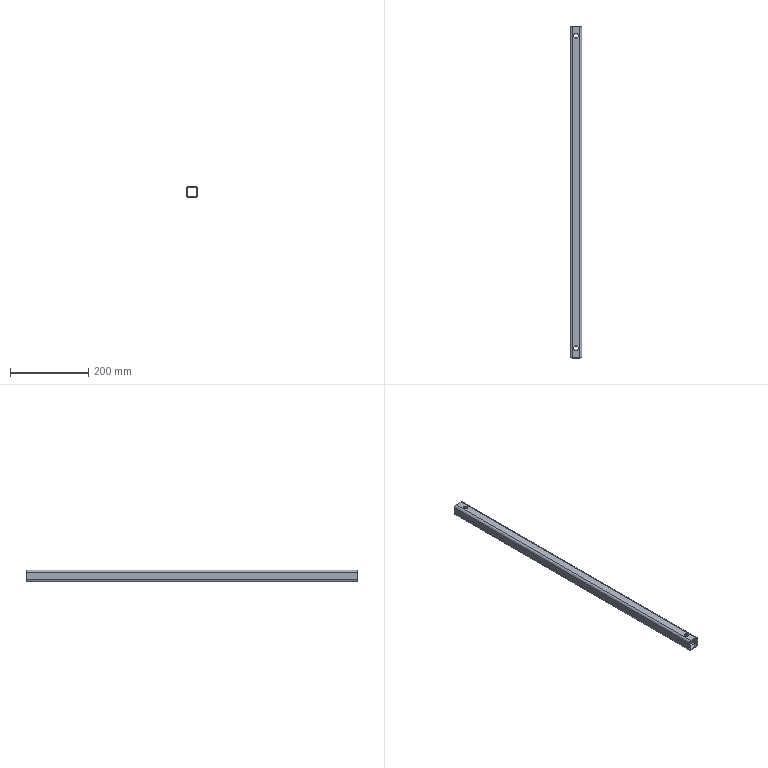Part | NX | features solid 2 | 1 solid | 30 faces | box 30 x 850 x 30 mm | volume 254291 mm3 | cylinder 16 | plane 14 | commonest cylinder face diameters 12 x12 6 x4
STEP:
#1=CARTESIAN_POINT('',(1092.,-720.,1295.));
#2=VERTEX_POINT('',#1);
#3=CARTESIAN_POINT('',(1092.,-720.,1298.));
#4=VERTEX_POINT('',#3);
#5=CARTESIAN_POINT('',(1092.,-720.,1325.));
#6=DIRECTION('',(0.,0.,-1.));
#7=VECTOR('',#6,1000.);
#8=LINE('',#5,#7);
#9=EDGE_CURVE('',#2,#4,#8,.F.);
#10=ORIENTED_EDGE('',*,*,#9,.T.);
#11=CARTESIAN_POINT('',(1104.,-720.,1298.));
#12=VERTEX_POINT('',#11);
#13=CARTESIAN_POINT('',(1098.,-720.,1298.));
#14=DIRECTION('',(0.,0.,-1.));
#15=DIRECTION('',(-1.,0.,0.));
#16=AXIS2_PLACEMENT_3D('',#13,#14,#15);
#17=CIRCLE('',#16,6.);
#18=EDGE_CURVE('',#12,#4,#17,.T.);
#19=ORIENTED_EDGE('',*,*,#18,.F.);
#20=CARTESIAN_POINT('',(1104.,-720.,1295.));
#21=VERTEX_POINT('',#20);
#22=CARTESIAN_POINT('',(1104.,-720.,1325.));
#23=DIRECTION('',(0.,0.,-1.));
#24=VECTOR('',#23,1000.);
#25=LINE('',#22,#24);
#26=EDGE_CURVE('',#12,#21,#25,.T.);
#27=ORIENTED_EDGE('',*,*,#26,.T.);
#28=CARTESIAN_POINT('',(1098.,-720.,1295.));
#29=DIRECTION('',(0.,0.,-1.));
#30=DIRECTION('',(-1.,0.,0.));
#31=AXIS2_PLACEMENT_3D('',#28,#29,#30);
#32=CIRCLE('',#31,6.);
#33=EDGE_CURVE('',#21,#2,#32,.T.);
#34=ORIENTED_EDGE('',*,*,#33,.T.);
#35=EDGE_LOOP('',(#10,#19,#27,#34));
#36=FACE_BOUND('',#35,.T.);
#37=CARTESIAN_POINT('',(1098.,-720.,1325.));
#38=DIRECTION('',(0.,0.,-1.));
#39=DIRECTION('',(1.,0.,0.));
#40=AXIS2_PLACEMENT_3D('',#37,#38,#39);
#41=CYLINDRICAL_SURFACE('',#40,6.);
#42=ADVANCED_FACE('',(#36),#41,.F.);
#43=CARTESIAN_POINT('',(1092.,-720.,1325.));
#44=VERTEX_POINT('',#43);
#45=CARTESIAN_POINT('',(1092.,-720.,1322.));
#46=VERTEX_POINT('',#45);
#47=CARTESIAN_POINT('',(1092.,-720.,1325.));
#48=DIRECTION('',(0.,0.,-1.));
#49=VECTOR('',#48,1000.);
#50=LINE('',#47,#49);
#51=EDGE_CURVE('',#44,#46,#50,.T.);
#52=ORIENTED_EDGE('',*,*,#51,.F.);
#53=CARTESIAN_POINT('',(1104.,-720.,1325.));
#54=VERTEX_POINT('',#53);
#55=CARTESIAN_POINT('',(1098.,-720.,1325.));
#56=DIRECTION('',(0.,0.,-1.));
#57=DIRECTION('',(1.,0.,0.));
#58=AXIS2_PLACEMENT_3D('',#55,#56,#57);
#59=CIRCLE('',#58,6.);
#60=EDGE_CURVE('',#54,#44,#59,.T.);
#61=ORIENTED_EDGE('',*,*,#60,.F.);
#62=CARTESIAN_POINT('',(1104.,-720.,1322.));
#63=VERTEX_POINT('',#62);
#64=CARTESIAN_POINT('',(1104.,-720.,1325.));
#65=DIRECTION('',(0.,0.,-1.));
#66=VECTOR('',#65,1000.);
#67=LINE('',#64,#66);
#68=EDGE_CURVE('',#63,#54,#67,.F.);
#69=ORIENTED_EDGE('',*,*,#68,.F.);
#70=CARTESIAN_POINT('',(1098.,-720.,1322.));
#71=DIRECTION('',(0.,0.,1.));
#72=DIRECTION('',(1.,0.,0.));
#73=AXIS2_PLACEMENT_3D('',#70,#71,#72);
#74=CIRCLE('',#73,6.);
#75=EDGE_CURVE('',#46,#63,#74,.T.);
#76=ORIENTED_EDGE('',*,*,#75,.F.);
#77=EDGE_LOOP('',(#52,#61,#69,#76));
#78=FACE_BOUND('',#77,.T.);
#79=CARTESIAN_POINT('',(1098.,-720.,1325.));
#80=DIRECTION('',(0.,0.,-1.));
#81=DIRECTION('',(1.,0.,0.));
#82=AXIS2_PLACEMENT_3D('',#79,#80,#81);
#83=CYLINDRICAL_SURFACE('',#82,6.);
#84=ADVANCED_FACE('',(#78),#83,.F.);
#85=CARTESIAN_POINT('',(1092.,-1520.,1295.));
#86=VERTEX_POINT('',#85);
#87=CARTESIAN_POINT('',(1092.,-1520.,1298.));
#88=VERTEX_POINT('',#87);
#89=CARTESIAN_POINT('',(1092.,-1520.,1325.));
#90=DIRECTION('',(0.,0.,-1.));
#91=VECTOR('',#90,1000.);
#92=LINE('',#89,#91);
#93=EDGE_CURVE('',#86,#88,#92,.F.);
#94=ORIENTED_EDGE('',*,*,#93,.T.);
#95=CARTESIAN_POINT('',(1104.,-1520.,1298.));
#96=VERTEX_POINT('',#95);
#97=CARTESIAN_POINT('',(1098.,-1520.,1298.));
#98=DIRECTION('',(0.,0.,-1.));
#99=DIRECTION('',(-1.,0.,0.));
#100=AXIS2_PLACEMENT_3D('',#97,#98,#99);
#101=CIRCLE('',#100,6.);
#102=EDGE_CURVE('',#96,#88,#101,.T.);
#103=ORIENTED_EDGE('',*,*,#102,.F.);
#104=CARTESIAN_POINT('',(1104.,-1520.,1295.));
#105=VERTEX_POINT('',#104);
#106=CARTESIAN_POINT('',(1104.,-1520.,1325.));
#107=DIRECTION('',(0.,0.,-1.));
#108=VECTOR('',#107,1000.);
#109=LINE('',#106,#108);
#110=EDGE_CURVE('',#96,#105,#109,.T.);
#111=ORIENTED_EDGE('',*,*,#110,.T.);
#112=CARTESIAN_POINT('',(1098.,-1520.,1295.));
#113=DIRECTION('',(0.,0.,-1.));
#114=DIRECTION('',(-1.,0.,0.));
#115=AXIS2_PLACEMENT_3D('',#112,#113,#114);
#116=CIRCLE('',#115,6.);
#117=EDGE_CURVE('',#105,#86,#116,.T.);
#118=ORIENTED_EDGE('',*,*,#117,.T.);
#119=EDGE_LOOP('',(#94,#103,#111,#118));
#120=FACE_BOUND('',#119,.T.);
#121=CARTESIAN_POINT('',(1098.,-1520.,1325.));
#122=DIRECTION('',(0.,0.,-1.));
#123=DIRECTION('',(1.,0.,0.));
#124=AXIS2_PLACEMENT_3D('',#121,#122,#123);
#125=CYLINDRICAL_SURFACE('',#124,6.);
#126=ADVANCED_FACE('',(#120),#125,.F.);
#127=CARTESIAN_POINT('',(1092.,-1520.,1325.));
#128=VERTEX_POINT('',#127);
#129=CARTESIAN_POINT('',(1092.,-1520.,1322.));
#130=VERTEX_POINT('',#129);
#131=CARTESIAN_POINT('',(1092.,-1520.,1325.));
#132=DIRECTION('',(0.,0.,-1.));
#133=VECTOR('',#132,1000.);
#134=LINE('',#131,#133);
#135=EDGE_CURVE('',#128,#130,#134,.T.);
#136=ORIENTED_EDGE('',*,*,#135,.F.);
#137=CARTESIAN_POINT('',(1104.,-1520.,1325.));
#138=VERTEX_POINT('',#137);
#139=CARTESIAN_POINT('',(1098.,-1520.,1325.));
#140=DIRECTION('',(0.,0.,-1.));
#141=DIRECTION('',(1.,0.,0.));
#142=AXIS2_PLACEMENT_3D('',#139,#140,#141);
#143=CIRCLE('',#142,6.);
#144=EDGE_CURVE('',#138,#128,#143,.T.);
#145=ORIENTED_EDGE('',*,*,#144,.F.);
#146=CARTESIAN_POINT('',(1104.,-1520.,1322.));
#147=VERTEX_POINT('',#146);
#148=CARTESIAN_POINT('',(1104.,-1520.,1325.));
#149=DIRECTION('',(0.,0.,-1.));
#150=VECTOR('',#149,1000.);
#151=LINE('',#148,#150);
#152=EDGE_CURVE('',#147,#138,#151,.F.);
#153=ORIENTED_EDGE('',*,*,#152,.F.);
#154=CARTESIAN_POINT('',(1098.,-1520.,1322.));
#155=DIRECTION('',(0.,0.,1.));
#156=DIRECTION('',(1.,0.,0.));
#157=AXIS2_PLACEMENT_3D('',#154,#155,#156);
#158=CIRCLE('',#157,6.);
#159=EDGE_CURVE('',#130,#147,#158,.T.);
#160=ORIENTED_EDGE('',*,*,#159,.F.);
#161=EDGE_LOOP('',(#136,#145,#153,#160));
#162=FACE_BOUND('',#161,.T.);
#163=CARTESIAN_POINT('',(1098.,-1520.,1325.));
#164=DIRECTION('',(0.,0.,-1.));
#165=DIRECTION('',(1.,0.,0.));
#166=AXIS2_PLACEMENT_3D('',#163,#164,#165);
#167=CYLINDRICAL_SURFACE('',#166,6.);
#168=ADVANCED_FACE('',(#162),#167,.F.);
#169=CARTESIAN_POINT('',(1110.,-695.,1319.));
#170=VERTEX_POINT('',#169);
#171=CARTESIAN_POINT('',(1110.,-695.,1310.01));
#172=VERTEX_POINT('',#171);
#173=CARTESIAN_POINT('',(1110.,-695.,1325.));
#174=DIRECTION('',(0.,0.,-1.));
#175=VECTOR('',#174,1000.);
#176=LINE('',#173,#175);
#177=EDGE_CURVE('',#170,#172,#176,.T.);
#178=ORIENTED_EDGE('',*,*,#177,.T.);
#179=CARTESIAN_POINT('',(1110.,-1545.,1310.01));
#180=VERTEX_POINT('',#179);
#181=CARTESIAN_POINT('',(1110.,-1545.,1310.01));
#182=DIRECTION('',(0.,1.,0.));
#183=VECTOR('',#182,1000.);
#184=LINE('',#181,#183);
#185=EDGE_CURVE('',#180,#172,#184,.T.);
#186=ORIENTED_EDGE('',*,*,#185,.F.);
#187=CARTESIAN_POINT('',(1110.,-1545.,1319.));
#188=VERTEX_POINT('',#187);
#189=CARTESIAN_POINT('',(1110.,-1545.,1325.));
#190=DIRECTION('',(0.,0.,-1.));
#191=VECTOR('',#190,1000.);
#192=LINE('',#189,#191);
#193=EDGE_CURVE('',#188,#180,#192,.T.);
#194=ORIENTED_EDGE('',*,*,#193,.F.);
#195=CARTESIAN_POINT('',(1110.,-1545.,1319.));
#196=DIRECTION('',(0.,1.,0.));
#197=VECTOR('',#196,1000.);
#198=LINE('',#195,#197);
#199=EDGE_CURVE('',#188,#170,#198,.T.);
#200=ORIENTED_EDGE('',*,*,#199,.T.);
#201=EDGE_LOOP('',(#178,#186,#194,#200));
#202=FACE_BOUND('',#201,.T.);
#203=CARTESIAN_POINT('',(1110.,-1545.,1325.));
#204=DIRECTION('',(1.,0.,0.));
#205=DIRECTION('',(0.,0.,-1.));
#206=AXIS2_PLACEMENT_3D('',#203,#204,#205);
#207=PLANE('',#206);
#208=ADVANCED_FACE('',(#202),#207,.F.);
#209=CARTESIAN_POINT('',(1107.,-695.,1322.));
#210=VERTEX_POINT('',#209);
#211=CARTESIAN_POINT('',(1107.,-695.,1319.));
#212=DIRECTION('',(0.,1.,0.));
#213=DIRECTION('',(-1.,0.,0.));
#214=AXIS2_PLACEMENT_3D('',#211,#212,#213);
#215=CIRCLE('',#214,3.);
#216=EDGE_CURVE('',#210,#170,#215,.T.);
#217=ORIENTED_EDGE('',*,*,#216,.T.);
#218=ORIENTED_EDGE('',*,*,#199,.F.);
#219=CARTESIAN_POINT('',(1107.,-1545.,1322.));
#220=VERTEX_POINT('',#219);
#221=CARTESIAN_POINT('',(1107.,-1545.,1319.));
#222=DIRECTION('',(0.,1.,0.));
#223=DIRECTION('',(-1.,0.,0.));
#224=AXIS2_PLACEMENT_3D('',#221,#222,#223);
#225=CIRCLE('',#224,3.);
#226=EDGE_CURVE('',#220,#188,#225,.T.);
#227=ORIENTED_EDGE('',*,*,#226,.F.);
#228=CARTESIAN_POINT('',(1107.,-1545.,1322.));
#229=DIRECTION('',(0.,1.,0.));
#230=VECTOR('',#229,1000.);
#231=LINE('',#228,#230);
#232=EDGE_CURVE('',#220,#210,#231,.T.);
#233=ORIENTED_EDGE('',*,*,#232,.T.);
#234=EDGE_LOOP('',(#217,#218,#227,#233));
#235=FACE_BOUND('',#234,.T.);
#236=CARTESIAN_POINT('',(1107.,-1545.,1319.));
#237=DIRECTION('',(0.,1.,0.));
#238=DIRECTION('',(-1.,0.,0.));
#239=AXIS2_PLACEMENT_3D('',#236,#237,#238);
#240=CYLINDRICAL_SURFACE('',#239,3.);
#241=ADVANCED_FACE('',(#235),#240,.F.);
#242=CARTESIAN_POINT('',(1098.,-1520.,1322.));
#243=DIRECTION('',(0.,0.,1.));
#244=DIRECTION('',(1.,0.,0.));
#245=AXIS2_PLACEMENT_3D('',#242,#243,#244);
#246=CIRCLE('',#245,6.);
#247=EDGE_CURVE('',#147,#130,#246,.T.);
#248=ORIENTED_EDGE('',*,*,#247,.T.);
#249=ORIENTED_EDGE('',*,*,#159,.T.);
#250=EDGE_LOOP('',(#248,#249));
#251=FACE_BOUND('',#250,.T.);
#252=CARTESIAN_POINT('',(1098.,-720.,1322.));
#253=DIRECTION('',(0.,0.,1.));
#254=DIRECTION('',(1.,0.,0.));
#255=AXIS2_PLACEMENT_3D('',#252,#253,#254);
#256=CIRCLE('',#255,6.);
#257=EDGE_CURVE('',#63,#46,#256,.T.);
#258=ORIENTED_EDGE('',*,*,#257,.T.);
#259=ORIENTED_EDGE('',*,*,#75,.T.);
#260=EDGE_LOOP('',(#258,#259));
#261=FACE_BOUND('',#260,.T.);
#262=CARTESIAN_POINT('',(1089.,-695.,1322.));
#263=VERTEX_POINT('',#262);
#264=CARTESIAN_POINT('',(1083.,-695.,1322.));
#265=DIRECTION('',(1.,0.,0.));
#266=VECTOR('',#265,1000.);
#267=LINE('',#264,#266);
#268=EDGE_CURVE('',#263,#210,#267,.T.);
#269=ORIENTED_EDGE('',*,*,#268,.T.);
#270=ORIENTED_EDGE('',*,*,#232,.F.);
#271=CARTESIAN_POINT('',(1089.,-1545.,1322.));
#272=VERTEX_POINT('',#271);
#273=CARTESIAN_POINT('',(1083.,-1545.,1322.));
#274=DIRECTION('',(1.,0.,0.));
#275=VECTOR('',#274,1000.);
#276=LINE('',#273,#275);
#277=EDGE_CURVE('',#272,#220,#276,.T.);
#278=ORIENTED_EDGE('',*,*,#277,.F.);
#279=CARTESIAN_POINT('',(1089.,-1545.,1322.));
#280=DIRECTION('',(0.,1.,0.));
#281=VECTOR('',#280,1000.);
#282=LINE('',#279,#281);
#283=EDGE_CURVE('',#272,#263,#282,.T.);
#284=ORIENTED_EDGE('',*,*,#283,.T.);
#285=EDGE_LOOP('',(#269,#270,#278,#284));
#286=FACE_BOUND('',#285,.T.);
#287=CARTESIAN_POINT('',(1083.,-1545.,1322.));
#288=DIRECTION('',(0.,0.,1.));
#289=DIRECTION('',(1.,0.,0.));
#290=AXIS2_PLACEMENT_3D('',#287,#288,#289);
#291=PLANE('',#290);
#292=ADVANCED_FACE('',(#251,#261,#286),#291,.F.);
#293=CARTESIAN_POINT('',(1086.,-695.,1319.));
#294=VERTEX_POINT('',#293);
#295=CARTESIAN_POINT('',(1089.,-695.,1319.));
#296=DIRECTION('',(0.,1.,0.));
#297=DIRECTION('',(-1.,0.,0.));
#298=AXIS2_PLACEMENT_3D('',#295,#296,#297);
#299=CIRCLE('',#298,3.);
#300=EDGE_CURVE('',#294,#263,#299,.T.);
#301=ORIENTED_EDGE('',*,*,#300,.T.);
#302=ORIENTED_EDGE('',*,*,#283,.F.);
#303=CARTESIAN_POINT('',(1086.,-1545.,1319.));
#304=VERTEX_POINT('',#303);
#305=CARTESIAN_POINT('',(1089.,-1545.,1319.));
#306=DIRECTION('',(0.,1.,0.));
#307=DIRECTION('',(-1.,0.,0.));
#308=AXIS2_PLACEMENT_3D('',#305,#306,#307);
#309=CIRCLE('',#308,3.);
#310=EDGE_CURVE('',#304,#272,#309,.T.);
#311=ORIENTED_EDGE('',*,*,#310,.F.);
#312=CARTESIAN_POINT('',(1086.,-1545.,1319.));
#313=DIRECTION('',(0.,1.,0.));
#314=VECTOR('',#313,1000.);
#315=LINE('',#312,#314);
#316=EDGE_CURVE('',#304,#294,#315,.T.);
#317=ORIENTED_EDGE('',*,*,#316,.T.);
#318=EDGE_LOOP('',(#301,#302,#311,#317));
#319=FACE_BOUND('',#318,.T.);
#320=CARTESIAN_POINT('',(1089.,-1545.,1319.));
#321=DIRECTION('',(0.,1.,0.));
#322=DIRECTION('',(-1.,0.,0.));
#323=AXIS2_PLACEMENT_3D('',#320,#321,#322);
#324=CYLINDRICAL_SURFACE('',#323,3.);
#325=ADVANCED_FACE('',(#319),#324,.F.);
#326=CARTESIAN_POINT('',(1086.,-695.,1301.));
#327=VERTEX_POINT('',#326);
#328=CARTESIAN_POINT('',(1086.,-695.,1295.));
#329=DIRECTION('',(0.,0.,1.));
#330=VECTOR('',#329,1000.);
#331=LINE('',#328,#330);
#332=EDGE_CURVE('',#327,#294,#331,.T.);
#333=ORIENTED_EDGE('',*,*,#332,.T.);
#334=ORIENTED_EDGE('',*,*,#316,.F.);
#335=CARTESIAN_POINT('',(1086.,-1545.,1301.));
#336=VERTEX_POINT('',#335);
#337=CARTESIAN_POINT('',(1086.,-1545.,1295.));
#338=DIRECTION('',(0.,0.,1.));
#339=VECTOR('',#338,1000.);
#340=LINE('',#337,#339);
#341=EDGE_CURVE('',#336,#304,#340,.T.);
#342=ORIENTED_EDGE('',*,*,#341,.F.);
#343=CARTESIAN_POINT('',(1086.,-1545.,1301.));
#344=DIRECTION('',(0.,1.,0.));
#345=VECTOR('',#344,1000.);
#346=LINE('',#343,#345);
#347=EDGE_CURVE('',#336,#327,#346,.T.);
#348=ORIENTED_EDGE('',*,*,#347,.T.);
#349=EDGE_LOOP('',(#333,#334,#342,#348));
#350=FACE_BOUND('',#349,.T.);
#351=CARTESIAN_POINT('',(1086.,-1545.,1295.));
#352=DIRECTION('',(-1.,0.,0.));
#353=DIRECTION('',(0.,0.,1.));
#354=AXIS2_PLACEMENT_3D('',#351,#352,#353);
#355=PLANE('',#354);
#356=ADVANCED_FACE('',(#350),#355,.F.);
#357=CARTESIAN_POINT('',(1089.,-695.,1298.));
#358=VERTEX_POINT('',#357);
#359=CARTESIAN_POINT('',(1089.,-695.,1301.));
#360=DIRECTION('',(0.,1.,0.));
#361=DIRECTION('',(-1.,0.,0.));
#362=AXIS2_PLACEMENT_3D('',#359,#360,#361);
#363=CIRCLE('',#362,3.);
#364=EDGE_CURVE('',#358,#327,#363,.T.);
#365=ORIENTED_EDGE('',*,*,#364,.T.);
#366=ORIENTED_EDGE('',*,*,#347,.F.);
#367=CARTESIAN_POINT('',(1089.,-1545.,1298.));
#368=VERTEX_POINT('',#367);
#369=CARTESIAN_POINT('',(1089.,-1545.,1301.));
#370=DIRECTION('',(0.,1.,0.));
#371=DIRECTION('',(-1.,0.,0.));
#372=AXIS2_PLACEMENT_3D('',#369,#370,#371);
#373=CIRCLE('',#372,3.);
#374=EDGE_CURVE('',#368,#336,#373,.T.);
#375=ORIENTED_EDGE('',*,*,#374,.F.);
#376=CARTESIAN_POINT('',(1089.,-1545.,1298.));
#377=DIRECTION('',(0.,1.,0.));
#378=VECTOR('',#377,1000.);
#379=LINE('',#376,#378);
#380=EDGE_CURVE('',#368,#358,#379,.T.);
#381=ORIENTED_EDGE('',*,*,#380,.T.);
#382=EDGE_LOOP('',(#365,#366,#375,#381));
#383=FACE_BOUND('',#382,.T.);
#384=CARTESIAN_POINT('',(1089.,-1545.,1301.));
#385=DIRECTION('',(0.,1.,0.));
#386=DIRECTION('',(-1.,0.,0.));
#387=AXIS2_PLACEMENT_3D('',#384,#385,#386);
#388=CYLINDRICAL_SURFACE('',#387,3.);
#389=ADVANCED_FACE('',(#383),#388,.F.);
#390=ORIENTED_EDGE('',*,*,#102,.T.);
#391=CARTESIAN_POINT('',(1098.,-1520.,1298.));
#392=DIRECTION('',(0.,0.,-1.));
#393=DIRECTION('',(-1.,0.,0.));
#394=AXIS2_PLACEMENT_3D('',#391,#392,#393);
#395=CIRCLE('',#394,6.);
#396=EDGE_CURVE('',#88,#96,#395,.T.);
#397=ORIENTED_EDGE('',*,*,#396,.T.);
#398=EDGE_LOOP('',(#390,#397));
#399=FACE_BOUND('',#398,.T.);
#400=ORIENTED_EDGE('',*,*,#18,.T.);
#401=CARTESIAN_POINT('',(1098.,-720.,1298.));
#402=DIRECTION('',(0.,0.,-1.));
#403=DIRECTION('',(-1.,0.,0.));
#404=AXIS2_PLACEMENT_3D('',#401,#402,#403);
#405=CIRCLE('',#404,6.);
#406=EDGE_CURVE('',#4,#12,#405,.T.);
#407=ORIENTED_EDGE('',*,*,#406,.T.);
#408=EDGE_LOOP('',(#400,#407));
#409=FACE_BOUND('',#408,.T.);
#410=CARTESIAN_POINT('',(1107.,-695.,1298.));
#411=VERTEX_POINT('',#410);
#412=CARTESIAN_POINT('',(1113.,-695.,1298.));
#413=DIRECTION('',(-1.,0.,0.));
#414=VECTOR('',#413,1000.);
#415=LINE('',#412,#414);
#416=EDGE_CURVE('',#411,#358,#415,.T.);
#417=ORIENTED_EDGE('',*,*,#416,.T.);
#418=ORIENTED_EDGE('',*,*,#380,.F.);
#419=CARTESIAN_POINT('',(1107.,-1545.,1298.));
#420=VERTEX_POINT('',#419);
#421=CARTESIAN_POINT('',(1113.,-1545.,1298.));
#422=DIRECTION('',(-1.,0.,0.));
#423=VECTOR('',#422,1000.);
#424=LINE('',#421,#423);
#425=EDGE_CURVE('',#420,#368,#424,.T.);
#426=ORIENTED_EDGE('',*,*,#425,.F.);
#427=CARTESIAN_POINT('',(1107.,-1545.,1298.));
#428=DIRECTION('',(0.,1.,0.));
#429=VECTOR('',#428,1000.);
#430=LINE('',#427,#429);
#431=EDGE_CURVE('',#420,#411,#430,.T.);
#432=ORIENTED_EDGE('',*,*,#431,.T.);
#433=EDGE_LOOP('',(#417,#418,#426,#432));
#434=FACE_BOUND('',#433,.T.);
#435=CARTESIAN_POINT('',(1113.,-1545.,1298.));
#436=DIRECTION('',(0.,0.,-1.));
#437=DIRECTION('',(0.,-1.,0.));
#438=AXIS2_PLACEMENT_3D('',#435,#436,#437);
#439=PLANE('',#438);
#440=ADVANCED_FACE('',(#399,#409,#434),#439,.F.);
#441=CARTESIAN_POINT('',(1110.,-695.,1301.));
#442=VERTEX_POINT('',#441);
#443=CARTESIAN_POINT('',(1107.,-695.,1301.));
#444=DIRECTION('',(0.,1.,0.));
#445=DIRECTION('',(-1.,0.,0.));
#446=AXIS2_PLACEMENT_3D('',#443,#444,#445);
#447=CIRCLE('',#446,3.);
#448=EDGE_CURVE('',#442,#411,#447,.T.);
#449=ORIENTED_EDGE('',*,*,#448,.T.);
#450=ORIENTED_EDGE('',*,*,#431,.F.);
#451=CARTESIAN_POINT('',(1110.,-1545.,1301.));
#452=VERTEX_POINT('',#451);
#453=CARTESIAN_POINT('',(1107.,-1545.,1301.));
#454=DIRECTION('',(0.,1.,0.));
#455=DIRECTION('',(-1.,0.,0.));
#456=AXIS2_PLACEMENT_3D('',#453,#454,#455);
#457=CIRCLE('',#456,3.);
#458=EDGE_CURVE('',#452,#420,#457,.T.);
#459=ORIENTED_EDGE('',*,*,#458,.F.);
#460=CARTESIAN_POINT('',(1110.,-1545.,1301.));
#461=DIRECTION('',(0.,1.,0.));
#462=VECTOR('',#461,1000.);
#463=LINE('',#460,#462);
#464=EDGE_CURVE('',#452,#442,#463,.T.);
#465=ORIENTED_EDGE('',*,*,#464,.T.);
#466=EDGE_LOOP('',(#449,#450,#459,#465));
#467=FACE_BOUND('',#466,.T.);
#468=CARTESIAN_POINT('',(1107.,-1545.,1301.));
#469=DIRECTION('',(0.,1.,0.));
#470=DIRECTION('',(-1.,0.,0.));
#471=AXIS2_PLACEMENT_3D('',#468,#469,#470);
#472=CYLINDRICAL_SURFACE('',#471,3.);
#473=ADVANCED_FACE('',(#467),#472,.F.);
#474=CARTESIAN_POINT('',(1110.,-695.,1309.99));
#475=VERTEX_POINT('',#474);
#476=CARTESIAN_POINT('',(1110.,-695.,1309.99));
#477=DIRECTION('',(0.,0.,-1.));
#478=VECTOR('',#477,1000.);
#479=LINE('',#476,#478);
#480=EDGE_CURVE('',#475,#442,#479,.T.);
#481=ORIENTED_EDGE('',*,*,#480,.T.);
#482=ORIENTED_EDGE('',*,*,#464,.F.);
#483=CARTESIAN_POINT('',(1110.,-1545.,1309.99));
#484=VERTEX_POINT('',#483);
#485=CARTESIAN_POINT('',(1110.,-1545.,1309.99));
#486=DIRECTION('',(0.,0.,-1.));
#487=VECTOR('',#486,1000.);
#488=LINE('',#485,#487);
#489=EDGE_CURVE('',#484,#452,#488,.T.);
#490=ORIENTED_EDGE('',*,*,#489,.F.);
#491=CARTESIAN_POINT('',(1110.,-1545.,1309.99));
#492=DIRECTION('',(0.,1.,0.));
#493=VECTOR('',#492,1000.);
#494=LINE('',#491,#493);
#495=EDGE_CURVE('',#484,#475,#494,.T.);
#496=ORIENTED_EDGE('',*,*,#495,.T.);
#497=EDGE_LOOP('',(#481,#482,#490,#496));
#498=FACE_BOUND('',#497,.T.);
#499=CARTESIAN_POINT('',(1110.,-1545.,1309.99));
#500=DIRECTION('',(1.,0.,0.));
#501=DIRECTION('',(0.,0.,1.));
#502=AXIS2_PLACEMENT_3D('',#499,#500,#501);
#503=PLANE('',#502);
#504=ADVANCED_FACE('',(#498),#503,.F.);
#505=CARTESIAN_POINT('',(1113.,-695.,1319.));
#506=VERTEX_POINT('',#505);
#507=CARTESIAN_POINT('',(1113.,-695.,1310.01));
#508=VERTEX_POINT('',#507);
#509=CARTESIAN_POINT('',(1113.,-695.,1325.));
#510=DIRECTION('',(0.,0.,-1.));
#511=VECTOR('',#510,1000.);
#512=LINE('',#509,#511);
#513=EDGE_CURVE('',#506,#508,#512,.T.);
#514=ORIENTED_EDGE('',*,*,#513,.F.);
#515=CARTESIAN_POINT('',(1113.,-1545.,1319.));
#516=VERTEX_POINT('',#515);
#517=CARTESIAN_POINT('',(1113.,-1545.,1319.));
#518=DIRECTION('',(0.,1.,0.));
#519=VECTOR('',#518,1000.);
#520=LINE('',#517,#519);
#521=EDGE_CURVE('',#516,#506,#520,.T.);
#522=ORIENTED_EDGE('',*,*,#521,.F.);
#523=CARTESIAN_POINT('',(1113.,-1545.,1310.01));
#524=VERTEX_POINT('',#523);
#525=CARTESIAN_POINT('',(1113.,-1545.,1325.));
#526=DIRECTION('',(0.,0.,-1.));
#527=VECTOR('',#526,1000.);
#528=LINE('',#525,#527);
#529=EDGE_CURVE('',#516,#524,#528,.T.);
#530=ORIENTED_EDGE('',*,*,#529,.T.);
#531=CARTESIAN_POINT('',(1113.,-1545.,1310.01));
#532=DIRECTION('',(0.,1.,0.));
#533=VECTOR('',#532,1000.);
#534=LINE('',#531,#533);
#535=EDGE_CURVE('',#524,#508,#534,.T.);
#536=ORIENTED_EDGE('',*,*,#535,.T.);
#537=EDGE_LOOP('',(#514,#522,#530,#536));
#538=FACE_BOUND('',#537,.T.);
#539=CARTESIAN_POINT('',(1113.,-1545.,1325.));
#540=DIRECTION('',(1.,0.,0.));
#541=DIRECTION('',(0.,0.,-1.));
#542=AXIS2_PLACEMENT_3D('',#539,#540,#541);
#543=PLANE('',#542);
#544=ADVANCED_FACE('',(#538),#543,.T.);
#545=CARTESIAN_POINT('',(1107.,-695.,1325.));
#546=VERTEX_POINT('',#545);
#547=CARTESIAN_POINT('',(1107.,-695.,1319.));
#548=DIRECTION('',(0.,1.,0.));
#549=DIRECTION('',(0.,0.,-1.));
#550=AXIS2_PLACEMENT_3D('',#547,#548,#549);
#551=CIRCLE('',#550,6.);
#552=EDGE_CURVE('',#546,#506,#551,.T.);
#553=ORIENTED_EDGE('',*,*,#552,.F.);
#554=CARTESIAN_POINT('',(1107.,-1545.,1325.));
#555=VERTEX_POINT('',#554);
#556=CARTESIAN_POINT('',(1107.,-1545.,1325.));
#557=DIRECTION('',(0.,1.,0.));
#558=VECTOR('',#557,1000.);
#559=LINE('',#556,#558);
#560=EDGE_CURVE('',#555,#546,#559,.T.);
#561=ORIENTED_EDGE('',*,*,#560,.F.);
#562=CARTESIAN_POINT('',(1107.,-1545.,1319.));
#563=DIRECTION('',(0.,1.,0.));
#564=DIRECTION('',(0.,0.,-1.));
#565=AXIS2_PLACEMENT_3D('',#562,#563,#564);
#566=CIRCLE('',#565,6.);
#567=EDGE_CURVE('',#555,#516,#566,.T.);
#568=ORIENTED_EDGE('',*,*,#567,.T.);
#569=ORIENTED_EDGE('',*,*,#521,.T.);
#570=EDGE_LOOP('',(#553,#561,#568,#569));
#571=FACE_BOUND('',#570,.T.);
#572=CARTESIAN_POINT('',(1107.,-1545.,1319.));
#573=DIRECTION('',(0.,1.,0.));
#574=DIRECTION('',(-1.,0.,0.));
#575=AXIS2_PLACEMENT_3D('',#572,#573,#574);
#576=CYLINDRICAL_SURFACE('',#575,6.);
#577=ADVANCED_FACE('',(#571),#576,.T.);
#578=ORIENTED_EDGE('',*,*,#144,.T.);
#579=CARTESIAN_POINT('',(1098.,-1520.,1325.));
#580=DIRECTION('',(0.,0.,-1.));
#581=DIRECTION('',(1.,0.,0.));
#582=AXIS2_PLACEMENT_3D('',#579,#580,#581);
#583=CIRCLE('',#582,6.);
#584=EDGE_CURVE('',#128,#138,#583,.T.);
#585=ORIENTED_EDGE('',*,*,#584,.T.);
#586=EDGE_LOOP('',(#578,#585));
#587=FACE_BOUND('',#586,.T.);
#588=ORIENTED_EDGE('',*,*,#60,.T.);
#589=CARTESIAN_POINT('',(1098.,-720.,1325.));
#590=DIRECTION('',(0.,0.,-1.));
#591=DIRECTION('',(1.,0.,0.));
#592=AXIS2_PLACEMENT_3D('',#589,#590,#591);
#593=CIRCLE('',#592,6.);
#594=EDGE_CURVE('',#44,#54,#593,.T.);
#595=ORIENTED_EDGE('',*,*,#594,.T.);
#596=EDGE_LOOP('',(#588,#595));
#597=FACE_BOUND('',#596,.T.);
#598=CARTESIAN_POINT('',(1089.,-695.,1325.));
#599=VERTEX_POINT('',#598);
#600=CARTESIAN_POINT('',(1083.,-695.,1325.));
#601=DIRECTION('',(1.,0.,0.));
#602=VECTOR('',#601,1000.);
#603=LINE('',#600,#602);
#604=EDGE_CURVE('',#599,#546,#603,.T.);
#605=ORIENTED_EDGE('',*,*,#604,.F.);
#606=CARTESIAN_POINT('',(1089.,-1545.,1325.));
#607=VERTEX_POINT('',#606);
#608=CARTESIAN_POINT('',(1089.,-1545.,1325.));
#609=DIRECTION('',(0.,1.,0.));
#610=VECTOR('',#609,1000.);
#611=LINE('',#608,#610);
#612=EDGE_CURVE('',#607,#599,#611,.T.);
#613=ORIENTED_EDGE('',*,*,#612,.F.);
#614=CARTESIAN_POINT('',(1083.,-1545.,1325.));
#615=DIRECTION('',(1.,0.,0.));
#616=VECTOR('',#615,1000.);
#617=LINE('',#614,#616);
#618=EDGE_CURVE('',#607,#555,#617,.T.);
#619=ORIENTED_EDGE('',*,*,#618,.T.);
#620=ORIENTED_EDGE('',*,*,#560,.T.);
#621=EDGE_LOOP('',(#605,#613,#619,#620));
#622=FACE_BOUND('',#621,.T.);
#623=CARTESIAN_POINT('',(1083.,-1545.,1325.));
#624=DIRECTION('',(0.,0.,1.));
#625=DIRECTION('',(1.,0.,0.));
#626=AXIS2_PLACEMENT_3D('',#623,#624,#625);
#627=PLANE('',#626);
#628=ADVANCED_FACE('',(#587,#597,#622),#627,.T.);
#629=CARTESIAN_POINT('',(1083.,-695.,1319.));
#630=VERTEX_POINT('',#629);
#631=CARTESIAN_POINT('',(1089.,-695.,1319.));
#632=DIRECTION('',(0.,1.,0.));
#633=DIRECTION('',(0.,0.,-1.));
#634=AXIS2_PLACEMENT_3D('',#631,#632,#633);
#635=CIRCLE('',#634,6.);
#636=EDGE_CURVE('',#630,#599,#635,.T.);
#637=ORIENTED_EDGE('',*,*,#636,.F.);
#638=CARTESIAN_POINT('',(1083.,-1545.,1319.));
#639=VERTEX_POINT('',#638);
#640=CARTESIAN_POINT('',(1083.,-1545.,1319.));
#641=DIRECTION('',(0.,1.,0.));
#642=VECTOR('',#641,1000.);
#643=LINE('',#640,#642);
#644=EDGE_CURVE('',#639,#630,#643,.T.);
#645=ORIENTED_EDGE('',*,*,#644,.F.);
#646=CARTESIAN_POINT('',(1089.,-1545.,1319.));
#647=DIRECTION('',(0.,1.,0.));
#648=DIRECTION('',(0.,0.,-1.));
#649=AXIS2_PLACEMENT_3D('',#646,#647,#648);
#650=CIRCLE('',#649,6.);
#651=EDGE_CURVE('',#639,#607,#650,.T.);
#652=ORIENTED_EDGE('',*,*,#651,.T.);
#653=ORIENTED_EDGE('',*,*,#612,.T.);
#654=EDGE_LOOP('',(#637,#645,#652,#653));
#655=FACE_BOUND('',#654,.T.);
#656=CARTESIAN_POINT('',(1089.,-1545.,1319.));
#657=DIRECTION('',(0.,1.,0.));
#658=DIRECTION('',(-1.,0.,0.));
#659=AXIS2_PLACEMENT_3D('',#656,#657,#658);
#660=CYLINDRICAL_SURFACE('',#659,6.);
#661=ADVANCED_FACE('',(#655),#660,.T.);
#662=CARTESIAN_POINT('',(1083.,-695.,1301.));
#663=VERTEX_POINT('',#662);
#664=CARTESIAN_POINT('',(1083.,-695.,1295.));
#665=DIRECTION('',(0.,0.,1.));
#666=VECTOR('',#665,1000.);
#667=LINE('',#664,#666);
#668=EDGE_CURVE('',#663,#630,#667,.T.);
#669=ORIENTED_EDGE('',*,*,#668,.F.);
#670=CARTESIAN_POINT('',(1083.,-1545.,1301.));
#671=VERTEX_POINT('',#670);
#672=CARTESIAN_POINT('',(1083.,-1545.,1301.));
#673=DIRECTION('',(0.,1.,0.));
#674=VECTOR('',#673,1000.);
#675=LINE('',#672,#674);
#676=EDGE_CURVE('',#671,#663,#675,.T.);
#677=ORIENTED_EDGE('',*,*,#676,.F.);
#678=CARTESIAN_POINT('',(1083.,-1545.,1295.));
#679=DIRECTION('',(0.,0.,1.));
#680=VECTOR('',#679,1000.);
#681=LINE('',#678,#680);
#682=EDGE_CURVE('',#671,#639,#681,.T.);
#683=ORIENTED_EDGE('',*,*,#682,.T.);
#684=ORIENTED_EDGE('',*,*,#644,.T.);
#685=EDGE_LOOP('',(#669,#677,#683,#684));
#686=FACE_BOUND('',#685,.T.);
#687=CARTESIAN_POINT('',(1083.,-1545.,1295.));
#688=DIRECTION('',(-1.,0.,0.));
#689=DIRECTION('',(0.,0.,1.));
#690=AXIS2_PLACEMENT_3D('',#687,#688,#689);
#691=PLANE('',#690);
#692=ADVANCED_FACE('',(#686),#691,.T.);
#693=CARTESIAN_POINT('',(1089.,-695.,1295.));
#694=VERTEX_POINT('',#693);
#695=CARTESIAN_POINT('',(1089.,-695.,1301.));
#696=DIRECTION('',(0.,1.,0.));
#697=DIRECTION('',(0.,0.,-1.));
#698=AXIS2_PLACEMENT_3D('',#695,#696,#697);
#699=CIRCLE('',#698,6.);
#700=EDGE_CURVE('',#694,#663,#699,.T.);
#701=ORIENTED_EDGE('',*,*,#700,.F.);
#702=CARTESIAN_POINT('',(1089.,-1545.,1295.));
#703=VERTEX_POINT('',#702);
#704=CARTESIAN_POINT('',(1089.,-1545.,1295.));
#705=DIRECTION('',(0.,1.,0.));
#706=VECTOR('',#705,1000.);
#707=LINE('',#704,#706);
#708=EDGE_CURVE('',#703,#694,#707,.T.);
#709=ORIENTED_EDGE('',*,*,#708,.F.);
#710=CARTESIAN_POINT('',(1089.,-1545.,1301.));
#711=DIRECTION('',(0.,1.,0.));
#712=DIRECTION('',(0.,0.,-1.));
#713=AXIS2_PLACEMENT_3D('',#710,#711,#712);
#714=CIRCLE('',#713,6.);
#715=EDGE_CURVE('',#703,#671,#714,.T.);
#716=ORIENTED_EDGE('',*,*,#715,.T.);
#717=ORIENTED_EDGE('',*,*,#676,.T.);
#718=EDGE_LOOP('',(#701,#709,#716,#717));
#719=FACE_BOUND('',#718,.T.);
#720=CARTESIAN_POINT('',(1089.,-1545.,1301.));
#721=DIRECTION('',(0.,1.,0.));
#722=DIRECTION('',(-1.,0.,0.));
#723=AXIS2_PLACEMENT_3D('',#720,#721,#722);
#724=CYLINDRICAL_SURFACE('',#723,6.);
#725=ADVANCED_FACE('',(#719),#724,.T.);
#726=ORIENTED_EDGE('',*,*,#117,.F.);
#727=CARTESIAN_POINT('',(1098.,-1520.,1295.));
#728=DIRECTION('',(0.,0.,-1.));
#729=DIRECTION('',(-1.,0.,0.));
#730=AXIS2_PLACEMENT_3D('',#727,#728,#729);
#731=CIRCLE('',#730,6.);
#732=EDGE_CURVE('',#86,#105,#731,.T.);
#733=ORIENTED_EDGE('',*,*,#732,.F.);
#734=EDGE_LOOP('',(#726,#733));
#735=FACE_BOUND('',#734,.T.);
#736=ORIENTED_EDGE('',*,*,#33,.F.);
#737=CARTESIAN_POINT('',(1098.,-720.,1295.));
#738=DIRECTION('',(0.,0.,-1.));
#739=DIRECTION('',(-1.,0.,0.));
#740=AXIS2_PLACEMENT_3D('',#737,#738,#739);
#741=CIRCLE('',#740,6.);
#742=EDGE_CURVE('',#2,#21,#741,.T.);
#743=ORIENTED_EDGE('',*,*,#742,.F.);
#744=EDGE_LOOP('',(#736,#743));
#745=FACE_BOUND('',#744,.T.);
#746=CARTESIAN_POINT('',(1107.,-695.,1295.));
#747=VERTEX_POINT('',#746);
#748=CARTESIAN_POINT('',(1113.,-695.,1295.));
#749=DIRECTION('',(-1.,0.,0.));
#750=VECTOR('',#749,1000.);
#751=LINE('',#748,#750);
#752=EDGE_CURVE('',#747,#694,#751,.T.);
#753=ORIENTED_EDGE('',*,*,#752,.F.);
#754=CARTESIAN_POINT('',(1107.,-1545.,1295.));
#755=VERTEX_POINT('',#754);
#756=CARTESIAN_POINT('',(1107.,-1545.,1295.));
#757=DIRECTION('',(0.,1.,0.));
#758=VECTOR('',#757,1000.);
#759=LINE('',#756,#758);
#760=EDGE_CURVE('',#755,#747,#759,.T.);
#761=ORIENTED_EDGE('',*,*,#760,.F.);
#762=CARTESIAN_POINT('',(1113.,-1545.,1295.));
#763=DIRECTION('',(-1.,0.,0.));
#764=VECTOR('',#763,1000.);
#765=LINE('',#762,#764);
#766=EDGE_CURVE('',#755,#703,#765,.T.);
#767=ORIENTED_EDGE('',*,*,#766,.T.);
#768=ORIENTED_EDGE('',*,*,#708,.T.);
#769=EDGE_LOOP('',(#753,#761,#767,#768));
#770=FACE_BOUND('',#769,.T.);
#771=CARTESIAN_POINT('',(1113.,-1545.,1295.));
#772=DIRECTION('',(0.,0.,-1.));
#773=DIRECTION('',(0.,-1.,0.));
#774=AXIS2_PLACEMENT_3D('',#771,#772,#773);
#775=PLANE('',#774);
#776=ADVANCED_FACE('',(#735,#745,#770),#775,.T.);
#777=CARTESIAN_POINT('',(1113.,-695.,1301.));
#778=VERTEX_POINT('',#777);
#779=CARTESIAN_POINT('',(1107.,-695.,1301.));
#780=DIRECTION('',(0.,1.,0.));
#781=DIRECTION('',(0.,0.,-1.));
#782=AXIS2_PLACEMENT_3D('',#779,#780,#781);
#783=CIRCLE('',#782,6.);
#784=EDGE_CURVE('',#778,#747,#783,.T.);
#785=ORIENTED_EDGE('',*,*,#784,.F.);
#786=CARTESIAN_POINT('',(1113.,-1545.,1301.));
#787=VERTEX_POINT('',#786);
#788=CARTESIAN_POINT('',(1113.,-1545.,1301.));
#789=DIRECTION('',(0.,1.,0.));
#790=VECTOR('',#789,1000.);
#791=LINE('',#788,#790);
#792=EDGE_CURVE('',#787,#778,#791,.T.);
#793=ORIENTED_EDGE('',*,*,#792,.F.);
#794=CARTESIAN_POINT('',(1107.,-1545.,1301.));
#795=DIRECTION('',(0.,1.,0.));
#796=DIRECTION('',(0.,0.,-1.));
#797=AXIS2_PLACEMENT_3D('',#794,#795,#796);
#798=CIRCLE('',#797,6.);
#799=EDGE_CURVE('',#787,#755,#798,.T.);
#800=ORIENTED_EDGE('',*,*,#799,.T.);
#801=ORIENTED_EDGE('',*,*,#760,.T.);
#802=EDGE_LOOP('',(#785,#793,#800,#801));
#803=FACE_BOUND('',#802,.T.);
#804=CARTESIAN_POINT('',(1107.,-1545.,1301.));
#805=DIRECTION('',(0.,1.,0.));
#806=DIRECTION('',(-1.,0.,0.));
#807=AXIS2_PLACEMENT_3D('',#804,#805,#806);
#808=CYLINDRICAL_SURFACE('',#807,6.);
#809=ADVANCED_FACE('',(#803),#808,.T.);
#810=CARTESIAN_POINT('',(1113.,-695.,1309.99));
#811=VERTEX_POINT('',#810);
#812=CARTESIAN_POINT('',(1113.,-695.,1309.99));
#813=DIRECTION('',(0.,0.,-1.));
#814=VECTOR('',#813,1000.);
#815=LINE('',#812,#814);
#816=EDGE_CURVE('',#811,#778,#815,.T.);
#817=ORIENTED_EDGE('',*,*,#816,.F.);
#818=CARTESIAN_POINT('',(1113.,-1545.,1309.99));
#819=VERTEX_POINT('',#818);
#820=CARTESIAN_POINT('',(1113.,-1545.,1309.99));
#821=DIRECTION('',(0.,1.,0.));
#822=VECTOR('',#821,1000.);
#823=LINE('',#820,#822);
#824=EDGE_CURVE('',#819,#811,#823,.T.);
#825=ORIENTED_EDGE('',*,*,#824,.F.);
#826=CARTESIAN_POINT('',(1113.,-1545.,1309.99));
#827=DIRECTION('',(0.,0.,-1.));
#828=VECTOR('',#827,1000.);
#829=LINE('',#826,#828);
#830=EDGE_CURVE('',#819,#787,#829,.T.);
#831=ORIENTED_EDGE('',*,*,#830,.T.);
#832=ORIENTED_EDGE('',*,*,#792,.T.);
#833=EDGE_LOOP('',(#817,#825,#831,#832));
#834=FACE_BOUND('',#833,.T.);
#835=CARTESIAN_POINT('',(1113.,-1545.,1309.99));
#836=DIRECTION('',(1.,0.,0.));
#837=DIRECTION('',(0.,0.,1.));
#838=AXIS2_PLACEMENT_3D('',#835,#836,#837);
#839=PLANE('',#838);
#840=ADVANCED_FACE('',(#834),#839,.T.);
#841=ORIENTED_EDGE('',*,*,#495,.F.);
#842=CARTESIAN_POINT('',(1113.,-1545.,1309.99));
#843=DIRECTION('',(1.,0.,0.));
#844=VECTOR('',#843,1000.);
#845=LINE('',#842,#844);
#846=EDGE_CURVE('',#484,#819,#845,.T.);
#847=ORIENTED_EDGE('',*,*,#846,.T.);
#848=ORIENTED_EDGE('',*,*,#824,.T.);
#849=CARTESIAN_POINT('',(1113.,-695.,1309.99));
#850=DIRECTION('',(1.,0.,0.));
#851=VECTOR('',#850,1000.);
#852=LINE('',#849,#851);
#853=EDGE_CURVE('',#475,#811,#852,.T.);
#854=ORIENTED_EDGE('',*,*,#853,.F.);
#855=EDGE_LOOP('',(#841,#847,#848,#854));
#856=FACE_BOUND('',#855,.T.);
#857=CARTESIAN_POINT('',(1113.,-1545.,1309.99));
#858=DIRECTION('',(0.,0.,-1.));
#859=DIRECTION('',(0.,-1.,0.));
#860=AXIS2_PLACEMENT_3D('',#857,#858,#859);
#861=PLANE('',#860);
#862=ADVANCED_FACE('',(#856),#861,.F.);
#863=ORIENTED_EDGE('',*,*,#816,.T.);
#864=ORIENTED_EDGE('',*,*,#784,.T.);
#865=ORIENTED_EDGE('',*,*,#752,.T.);
#866=ORIENTED_EDGE('',*,*,#700,.T.);
#867=ORIENTED_EDGE('',*,*,#668,.T.);
#868=ORIENTED_EDGE('',*,*,#636,.T.);
#869=ORIENTED_EDGE('',*,*,#604,.T.);
#870=ORIENTED_EDGE('',*,*,#552,.T.);
#871=ORIENTED_EDGE('',*,*,#513,.T.);
#872=CARTESIAN_POINT('',(1113.,-695.,1310.01));
#873=DIRECTION('',(1.,0.,0.));
#874=VECTOR('',#873,1000.);
#875=LINE('',#872,#874);
#876=EDGE_CURVE('',#172,#508,#875,.T.);
#877=ORIENTED_EDGE('',*,*,#876,.F.);
#878=ORIENTED_EDGE('',*,*,#177,.F.);
#879=ORIENTED_EDGE('',*,*,#216,.F.);
#880=ORIENTED_EDGE('',*,*,#268,.F.);
#881=ORIENTED_EDGE('',*,*,#300,.F.);
#882=ORIENTED_EDGE('',*,*,#332,.F.);
#883=ORIENTED_EDGE('',*,*,#364,.F.);
#884=ORIENTED_EDGE('',*,*,#416,.F.);
#885=ORIENTED_EDGE('',*,*,#448,.F.);
#886=ORIENTED_EDGE('',*,*,#480,.F.);
#887=ORIENTED_EDGE('',*,*,#853,.T.);
#888=EDGE_LOOP('',(#863,#864,#865,#866,#867,#868,#869,#870,#871,#877,#878,#879,#880,#881,#882,#883,#884,#885,#886,#887));
#889=FACE_BOUND('',#888,.T.);
#890=CARTESIAN_POINT('',(1113.,-695.,1309.99));
#891=DIRECTION('',(0.,-1.,0.));
#892=DIRECTION('',(-1.,0.,0.));
#893=AXIS2_PLACEMENT_3D('',#890,#891,#892);
#894=PLANE('',#893);
#895=ADVANCED_FACE('',(#889),#894,.F.);
#896=CARTESIAN_POINT('',(1113.,-1545.,1310.01));
#897=DIRECTION('',(1.,0.,0.));
#898=VECTOR('',#897,1000.);
#899=LINE('',#896,#898);
#900=EDGE_CURVE('',#180,#524,#899,.T.);
#901=ORIENTED_EDGE('',*,*,#900,.F.);
#902=ORIENTED_EDGE('',*,*,#185,.T.);
#903=ORIENTED_EDGE('',*,*,#876,.T.);
#904=ORIENTED_EDGE('',*,*,#535,.F.);
#905=EDGE_LOOP('',(#901,#902,#903,#904));
#906=FACE_BOUND('',#905,.T.);
#907=CARTESIAN_POINT('',(1113.,-1545.,1310.01));
#908=DIRECTION('',(0.,0.,-1.));
#909=DIRECTION('',(-1.,0.,0.));
#910=AXIS2_PLACEMENT_3D('',#907,#908,#909);
#911=PLANE('',#910);
#912=ADVANCED_FACE('',(#906),#911,.T.);
#913=ORIENTED_EDGE('',*,*,#529,.F.);
#914=ORIENTED_EDGE('',*,*,#567,.F.);
#915=ORIENTED_EDGE('',*,*,#618,.F.);
#916=ORIENTED_EDGE('',*,*,#651,.F.);
#917=ORIENTED_EDGE('',*,*,#682,.F.);
#918=ORIENTED_EDGE('',*,*,#715,.F.);
#919=ORIENTED_EDGE('',*,*,#766,.F.);
#920=ORIENTED_EDGE('',*,*,#799,.F.);
#921=ORIENTED_EDGE('',*,*,#830,.F.);
#922=ORIENTED_EDGE('',*,*,#846,.F.);
#923=ORIENTED_EDGE('',*,*,#489,.T.);
#924=ORIENTED_EDGE('',*,*,#458,.T.);
#925=ORIENTED_EDGE('',*,*,#425,.T.);
#926=ORIENTED_EDGE('',*,*,#374,.T.);
#927=ORIENTED_EDGE('',*,*,#341,.T.);
#928=ORIENTED_EDGE('',*,*,#310,.T.);
#929=ORIENTED_EDGE('',*,*,#277,.T.);
#930=ORIENTED_EDGE('',*,*,#226,.T.);
#931=ORIENTED_EDGE('',*,*,#193,.T.);
#932=ORIENTED_EDGE('',*,*,#900,.T.);
#933=EDGE_LOOP('',(#913,#914,#915,#916,#917,#918,#919,#920,#921,#922,#923,#924,#925,#926,#927,#928,#929,#930,#931,#932));
#934=FACE_BOUND('',#933,.T.);
#935=CARTESIAN_POINT('',(1113.,-1545.,1325.));
#936=DIRECTION('',(0.,-1.,0.));
#937=DIRECTION('',(-1.,0.,0.));
#938=AXIS2_PLACEMENT_3D('',#935,#936,#937);
#939=PLANE('',#938);
#940=ADVANCED_FACE('',(#934),#939,.T.);
#941=ORIENTED_EDGE('',*,*,#584,.F.);
#942=ORIENTED_EDGE('',*,*,#135,.T.);
#943=ORIENTED_EDGE('',*,*,#247,.F.);
#944=ORIENTED_EDGE('',*,*,#152,.T.);
#945=EDGE_LOOP('',(#941,#942,#943,#944));
#946=FACE_BOUND('',#945,.T.);
#947=CARTESIAN_POINT('',(1098.,-1520.,1325.));
#948=DIRECTION('',(0.,0.,-1.));
#949=DIRECTION('',(1.,0.,0.));
#950=AXIS2_PLACEMENT_3D('',#947,#948,#949);
#951=CYLINDRICAL_SURFACE('',#950,6.);
#952=ADVANCED_FACE('',(#946),#951,.F.);
#953=ORIENTED_EDGE('',*,*,#396,.F.);
#954=ORIENTED_EDGE('',*,*,#93,.F.);
#955=ORIENTED_EDGE('',*,*,#732,.T.);
#956=ORIENTED_EDGE('',*,*,#110,.F.);
#957=EDGE_LOOP('',(#953,#954,#955,#956));
#958=FACE_BOUND('',#957,.T.);
#959=CARTESIAN_POINT('',(1098.,-1520.,1325.));
#960=DIRECTION('',(0.,0.,-1.));
#961=DIRECTION('',(1.,0.,0.));
#962=AXIS2_PLACEMENT_3D('',#959,#960,#961);
#963=CYLINDRICAL_SURFACE('',#962,6.);
#964=ADVANCED_FACE('',(#958),#963,.F.);
#965=ORIENTED_EDGE('',*,*,#594,.F.);
#966=ORIENTED_EDGE('',*,*,#51,.T.);
#967=ORIENTED_EDGE('',*,*,#257,.F.);
#968=ORIENTED_EDGE('',*,*,#68,.T.);
#969=EDGE_LOOP('',(#965,#966,#967,#968));
#970=FACE_BOUND('',#969,.T.);
#971=CARTESIAN_POINT('',(1098.,-720.,1325.));
#972=DIRECTION('',(0.,0.,-1.));
#973=DIRECTION('',(1.,0.,0.));
#974=AXIS2_PLACEMENT_3D('',#971,#972,#973);
#975=CYLINDRICAL_SURFACE('',#974,6.);
#976=ADVANCED_FACE('',(#970),#975,.F.);
#977=ORIENTED_EDGE('',*,*,#406,.F.);
#978=ORIENTED_EDGE('',*,*,#9,.F.);
#979=ORIENTED_EDGE('',*,*,#742,.T.);
#980=ORIENTED_EDGE('',*,*,#26,.F.);
#981=EDGE_LOOP('',(#977,#978,#979,#980));
#982=FACE_BOUND('',#981,.T.);
#983=CARTESIAN_POINT('',(1098.,-720.,1325.));
#984=DIRECTION('',(0.,0.,-1.));
#985=DIRECTION('',(1.,0.,0.));
#986=AXIS2_PLACEMENT_3D('',#983,#984,#985);
#987=CYLINDRICAL_SURFACE('',#986,6.);
#988=ADVANCED_FACE('',(#982),#987,.F.);
#989=CLOSED_SHELL('',(#42,#84,#126,#168,#208,#241,#292,#325,#356,#389,#440,#473,#504,#544,#577,#628,#661,#692,#725,#776,#809,#840,#862,#895,#912,#940,#952,#964,#976,#988));
#990=MANIFOLD_SOLID_BREP('',#989);
#991=(LENGTH_UNIT()NAMED_UNIT(*)SI_UNIT(.MILLI.,.METRE.));
#992=UNCERTAINTY_MEASURE_WITH_UNIT(LENGTH_MEASURE(0.00001),#991,'','');
#993=(NAMED_UNIT(*)PLANE_ANGLE_UNIT()SI_UNIT($,.RADIAN.));
#994=(NAMED_UNIT(*)SI_UNIT($,.STERADIAN.)SOLID_ANGLE_UNIT());
#995=(GEOMETRIC_REPRESENTATION_CONTEXT(3)GLOBAL_UNCERTAINTY_ASSIGNED_CONTEXT((#992))GLOBAL_UNIT_ASSIGNED_CONTEXT((#991,#993,#994))REPRESENTATION_CONTEXT('',''));
#996=ADVANCED_BREP_SHAPE_REPRESENTATION('',(#990),#995);